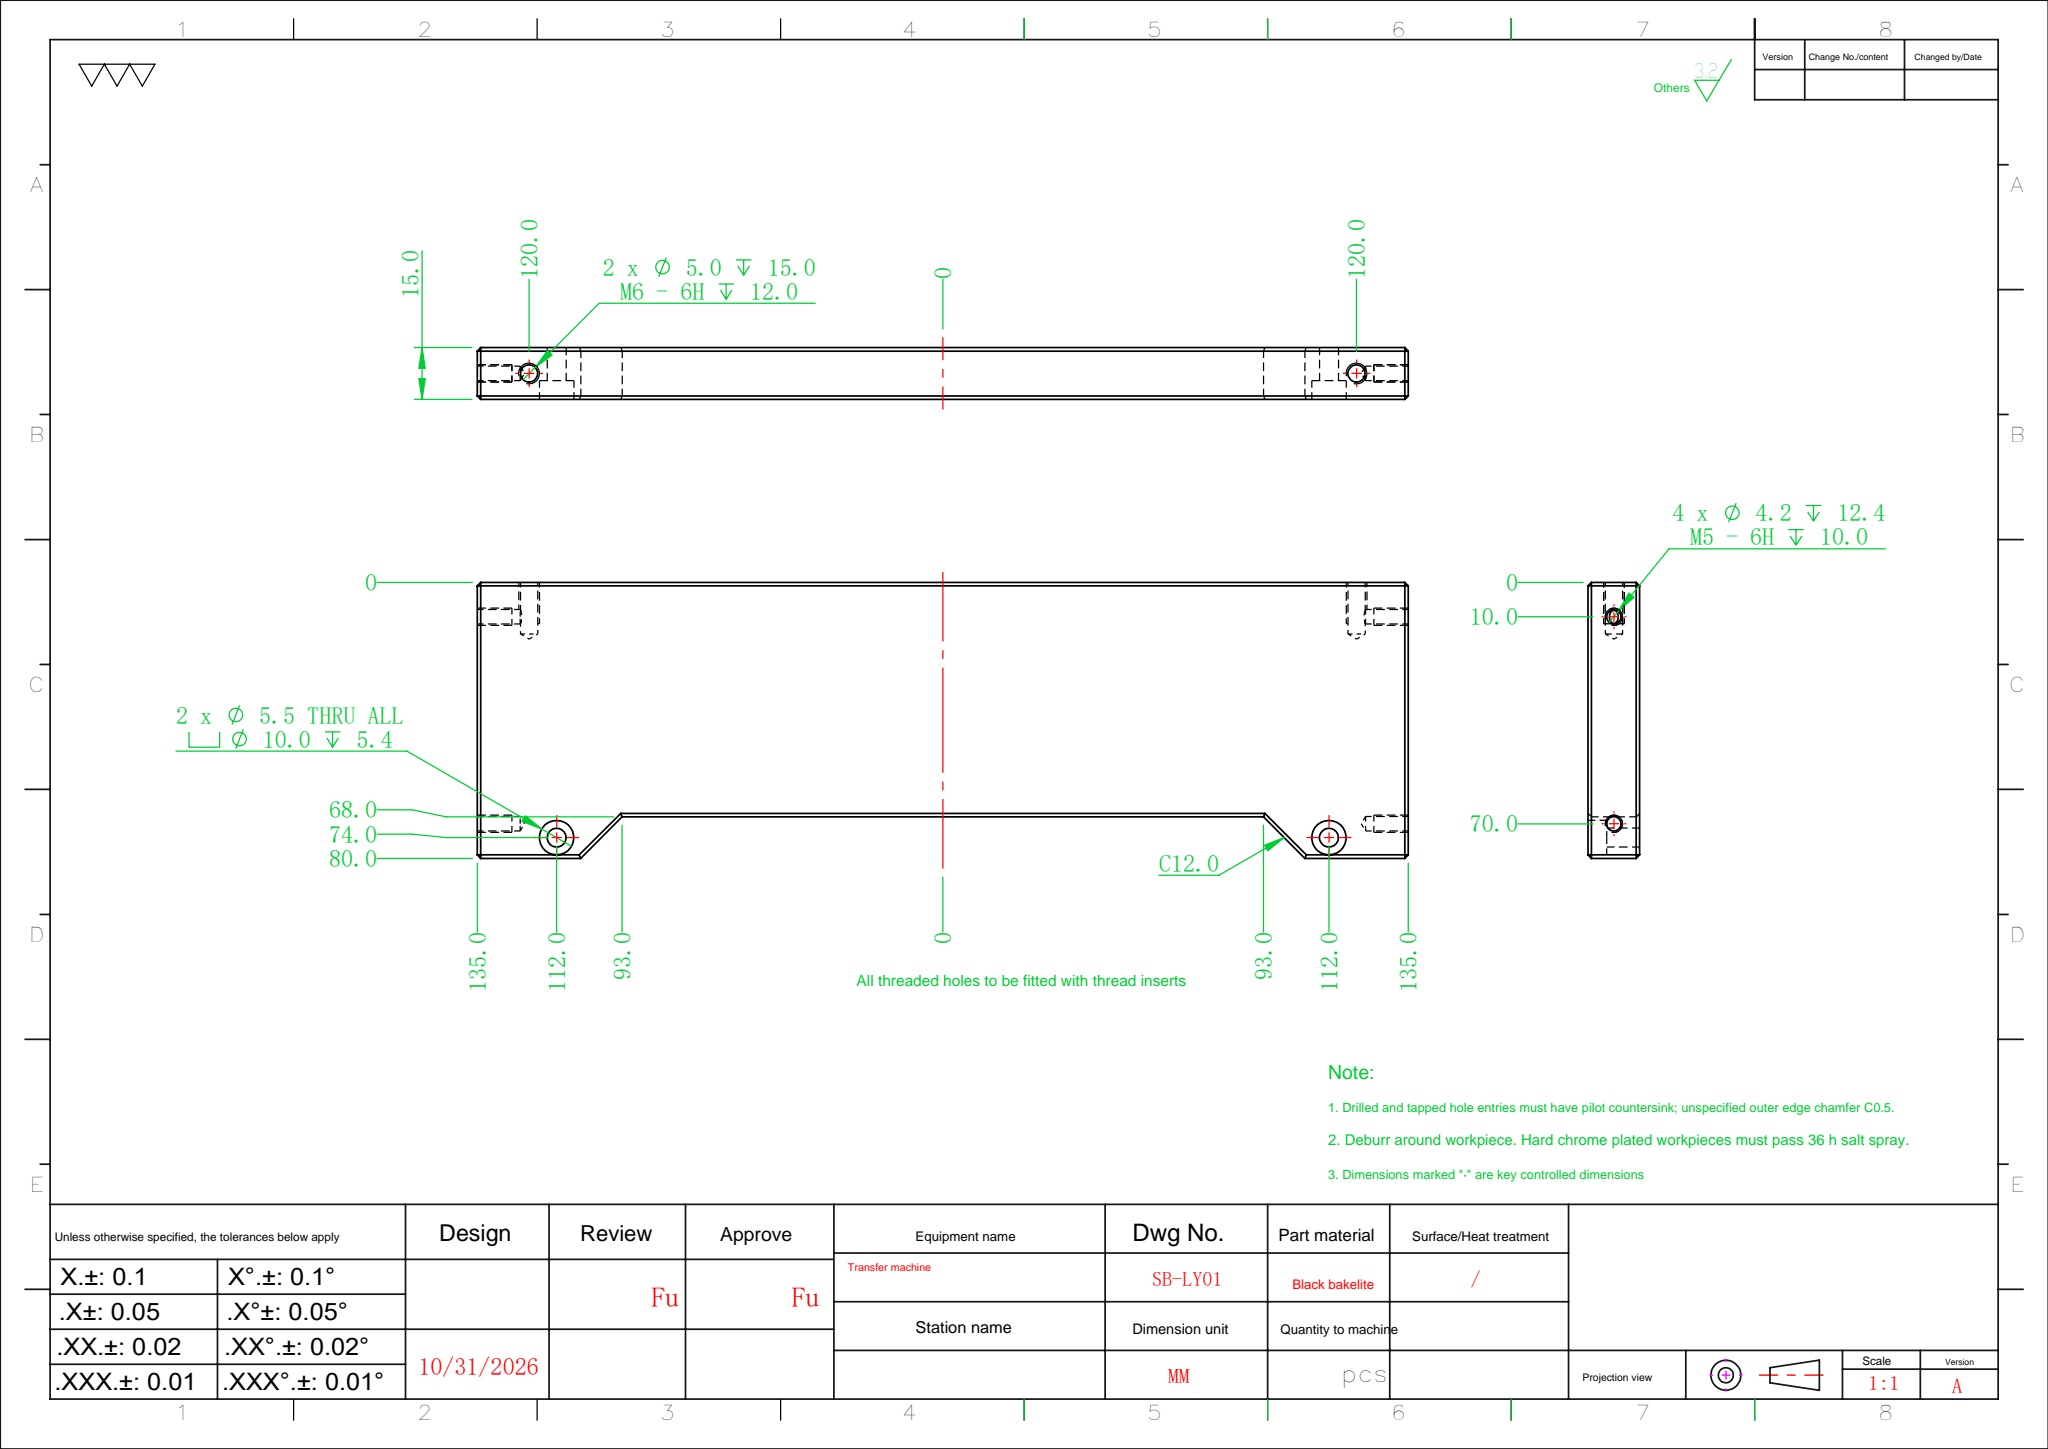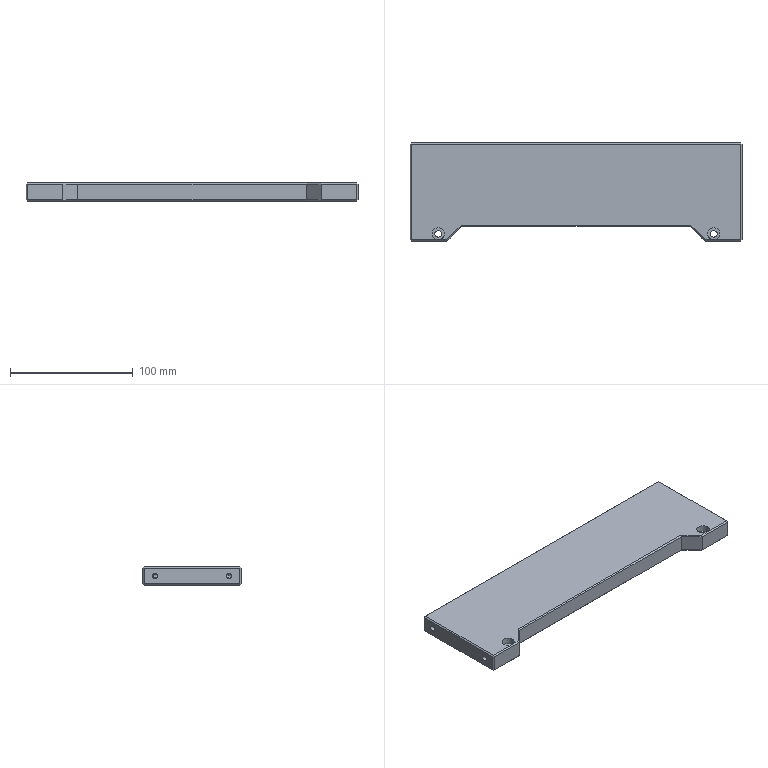Part | SolidWorks | features HoleWzd 3, Chamfer 2, Cut 1, Extrusion 1, MirrorPattern 1 | 1 solid | 72 faces | box 270 x 80 x 15 mm | volume 285008 mm3 | plane 40 | cylinder 20 | cone 12 | commonest cylinder face diameters 4.2 x8 5 x4 5.5 x4 10 x4